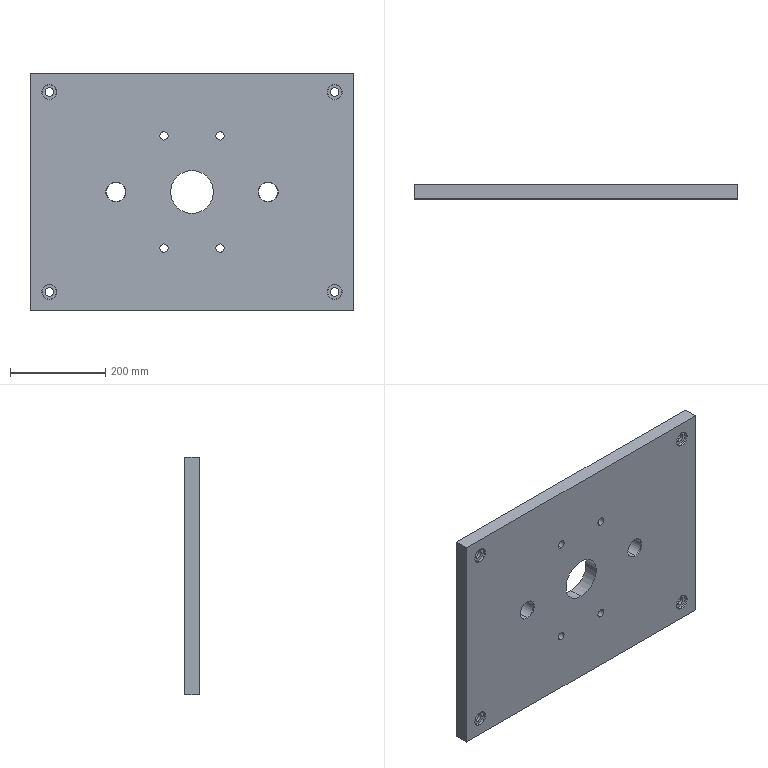Part | STEP file | OP10-017_upper plate (L) | 1 solid | 100 faces | box 680 x 30 x 500 mm | volume 9842603 mm3 | cylinder 54 | cone 32 | plane 14 | commonest cylinder face diameters 4.2 x16 17.5 x8 18 x8 26 x8 30 x8 40 x4